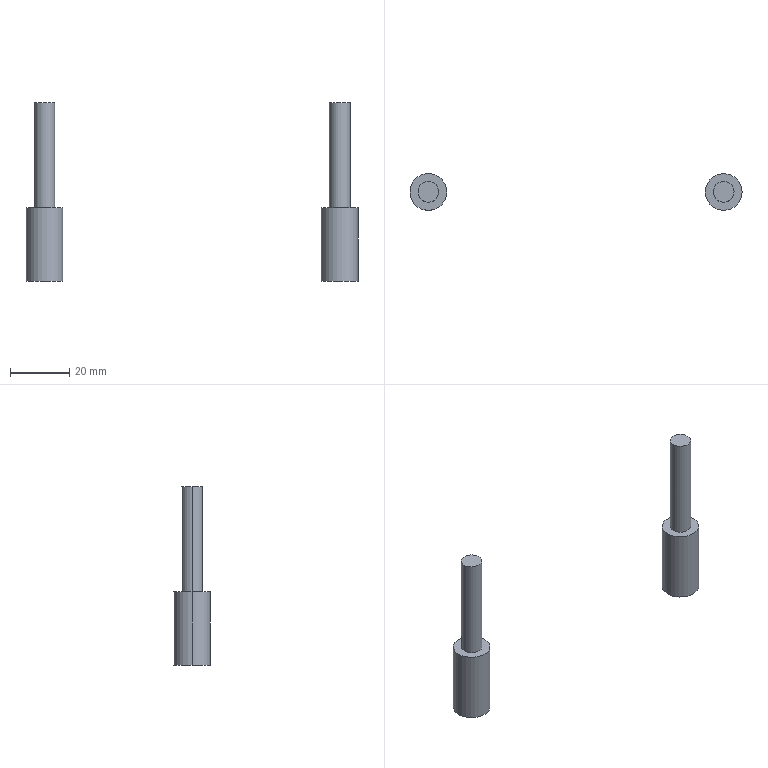Part | STEP file | 吸盘导柱-2 | 2 solids | 14 faces | box 112.418 x 12.438 x 60.6 mm | volume 8796 mm3 | cylinder 8 | plane 6 | commonest cylinder face diameters 7 x4 12.399 x2 12.438 x2
STEP:
#1=CARTESIAN_POINT('',(3.5,0.,60.6));
#2=VERTEX_POINT('',#1);
#3=CARTESIAN_POINT('',(-3.5,0.,60.6));
#4=VERTEX_POINT('',#3);
#5=CARTESIAN_POINT('',(0.,0.,60.6));
#6=DIRECTION('',(0.,0.,1.));
#7=DIRECTION('',(1.,0.,0.));
#8=AXIS2_PLACEMENT_3D('',#5,#6,#7);
#9=CIRCLE('',#8,3.5);
#10=EDGE_CURVE('',#2,#4,#9,.T.);
#11=ORIENTED_EDGE('',*,*,#10,.F.);
#12=CARTESIAN_POINT('',(3.5,0.,25.));
#13=VERTEX_POINT('',#12);
#14=CARTESIAN_POINT('',(3.5,0.,60.6));
#15=DIRECTION('',(0.,0.,-1.));
#16=VECTOR('',#15,1000.);
#17=LINE('',#14,#16);
#18=EDGE_CURVE('',#2,#13,#17,.T.);
#19=ORIENTED_EDGE('',*,*,#18,.T.);
#20=CARTESIAN_POINT('',(-3.5,0.,25.));
#21=VERTEX_POINT('',#20);
#22=CARTESIAN_POINT('',(0.,0.,25.));
#23=DIRECTION('',(0.,0.,1.));
#24=DIRECTION('',(1.,0.,0.));
#25=AXIS2_PLACEMENT_3D('',#22,#23,#24);
#26=CIRCLE('',#25,3.5);
#27=EDGE_CURVE('',#13,#21,#26,.T.);
#28=ORIENTED_EDGE('',*,*,#27,.T.);
#29=CARTESIAN_POINT('',(-3.5,0.,60.6));
#30=DIRECTION('',(0.,0.,-1.));
#31=VECTOR('',#30,1000.);
#32=LINE('',#29,#31);
#33=EDGE_CURVE('',#4,#21,#32,.T.);
#34=ORIENTED_EDGE('',*,*,#33,.F.);
#35=EDGE_LOOP('',(#11,#19,#28,#34));
#36=FACE_OUTER_BOUND('',#35,.T.);
#37=CARTESIAN_POINT('',(0.,0.,60.6));
#38=DIRECTION('',(0.,0.,-1.));
#39=DIRECTION('',(-1.,0.,0.));
#40=AXIS2_PLACEMENT_3D('',#37,#38,#39);
#41=CYLINDRICAL_SURFACE('',#40,3.5);
#42=ADVANCED_FACE('',(#36),#41,.T.);
#43=CARTESIAN_POINT('',(6.219,0.,25.));
#44=VERTEX_POINT('',#43);
#45=CARTESIAN_POINT('',(-6.219,0.,25.));
#46=VERTEX_POINT('',#45);
#47=CARTESIAN_POINT('',(0.,0.,25.));
#48=DIRECTION('',(0.,0.,1.));
#49=DIRECTION('',(1.,0.,0.));
#50=AXIS2_PLACEMENT_3D('',#47,#48,#49);
#51=CIRCLE('',#50,6.219);
#52=EDGE_CURVE('',#44,#46,#51,.T.);
#53=ORIENTED_EDGE('',*,*,#52,.F.);
#54=CARTESIAN_POINT('',(6.219,0.,0.));
#55=VERTEX_POINT('',#54);
#56=CARTESIAN_POINT('',(6.219,0.,25.));
#57=DIRECTION('',(0.,0.,-1.));
#58=VECTOR('',#57,1000.);
#59=LINE('',#56,#58);
#60=EDGE_CURVE('',#44,#55,#59,.T.);
#61=ORIENTED_EDGE('',*,*,#60,.T.);
#62=CARTESIAN_POINT('',(-6.219,0.,0.));
#63=VERTEX_POINT('',#62);
#64=CARTESIAN_POINT('',(0.,0.,0.));
#65=DIRECTION('',(0.,0.,1.));
#66=DIRECTION('',(1.,0.,0.));
#67=AXIS2_PLACEMENT_3D('',#64,#65,#66);
#68=CIRCLE('',#67,6.219);
#69=EDGE_CURVE('',#55,#63,#68,.T.);
#70=ORIENTED_EDGE('',*,*,#69,.T.);
#71=CARTESIAN_POINT('',(-6.219,0.,25.));
#72=DIRECTION('',(0.,0.,-1.));
#73=VECTOR('',#72,1000.);
#74=LINE('',#71,#73);
#75=EDGE_CURVE('',#46,#63,#74,.T.);
#76=ORIENTED_EDGE('',*,*,#75,.F.);
#77=EDGE_LOOP('',(#53,#61,#70,#76));
#78=FACE_OUTER_BOUND('',#77,.T.);
#79=CARTESIAN_POINT('',(0.,0.,25.));
#80=DIRECTION('',(0.,0.,-1.));
#81=DIRECTION('',(-1.,0.,0.));
#82=AXIS2_PLACEMENT_3D('',#79,#80,#81);
#83=CYLINDRICAL_SURFACE('',#82,6.219);
#84=ADVANCED_FACE('',(#78),#83,.T.);
#85=CARTESIAN_POINT('',(0.,0.,25.));
#86=DIRECTION('',(0.,0.,1.));
#87=DIRECTION('',(1.,0.,0.));
#88=AXIS2_PLACEMENT_3D('',#85,#86,#87);
#89=CIRCLE('',#88,6.219);
#90=EDGE_CURVE('',#46,#44,#89,.T.);
#91=ORIENTED_EDGE('',*,*,#90,.T.);
#92=ORIENTED_EDGE('',*,*,#52,.T.);
#93=EDGE_LOOP('',(#91,#92));
#94=FACE_OUTER_BOUND('',#93,.T.);
#95=CARTESIAN_POINT('',(0.,0.,25.));
#96=DIRECTION('',(0.,0.,1.));
#97=DIRECTION('',(1.,0.,0.));
#98=AXIS2_PLACEMENT_3D('',#95,#96,#97);
#99=CIRCLE('',#98,3.5);
#100=EDGE_CURVE('',#21,#13,#99,.T.);
#101=ORIENTED_EDGE('',*,*,#100,.F.);
#102=ORIENTED_EDGE('',*,*,#27,.F.);
#103=EDGE_LOOP('',(#101,#102));
#104=FACE_BOUND('',#103,.T.);
#105=CARTESIAN_POINT('',(0.,0.,25.));
#106=DIRECTION('',(0.,0.,1.));
#107=DIRECTION('',(1.,0.,0.));
#108=AXIS2_PLACEMENT_3D('',#105,#106,#107);
#109=PLANE('',#108);
#110=ADVANCED_FACE('',(#94,#104),#109,.T.);
#111=ORIENTED_EDGE('',*,*,#60,.F.);
#112=ORIENTED_EDGE('',*,*,#90,.F.);
#113=ORIENTED_EDGE('',*,*,#75,.T.);
#114=CARTESIAN_POINT('',(0.,0.,0.));
#115=DIRECTION('',(0.,0.,1.));
#116=DIRECTION('',(1.,0.,0.));
#117=AXIS2_PLACEMENT_3D('',#114,#115,#116);
#118=CIRCLE('',#117,6.219);
#119=EDGE_CURVE('',#63,#55,#118,.T.);
#120=ORIENTED_EDGE('',*,*,#119,.T.);
#121=EDGE_LOOP('',(#111,#112,#113,#120));
#122=FACE_OUTER_BOUND('',#121,.T.);
#123=CARTESIAN_POINT('',(0.,0.,25.));
#124=DIRECTION('',(0.,0.,-1.));
#125=DIRECTION('',(-1.,0.,0.));
#126=AXIS2_PLACEMENT_3D('',#123,#124,#125);
#127=CYLINDRICAL_SURFACE('',#126,6.219);
#128=ADVANCED_FACE('',(#122),#127,.T.);
#129=ORIENTED_EDGE('',*,*,#119,.F.);
#130=ORIENTED_EDGE('',*,*,#69,.F.);
#131=EDGE_LOOP('',(#129,#130));
#132=FACE_OUTER_BOUND('',#131,.T.);
#133=CARTESIAN_POINT('',(0.,0.,0.));
#134=DIRECTION('',(0.,0.,1.));
#135=DIRECTION('',(1.,0.,0.));
#136=AXIS2_PLACEMENT_3D('',#133,#134,#135);
#137=PLANE('',#136);
#138=ADVANCED_FACE('',(#132),#137,.F.);
#139=ORIENTED_EDGE('',*,*,#18,.F.);
#140=CARTESIAN_POINT('',(0.,0.,60.6));
#141=DIRECTION('',(0.,0.,1.));
#142=DIRECTION('',(1.,0.,0.));
#143=AXIS2_PLACEMENT_3D('',#140,#141,#142);
#144=CIRCLE('',#143,3.5);
#145=EDGE_CURVE('',#4,#2,#144,.T.);
#146=ORIENTED_EDGE('',*,*,#145,.F.);
#147=ORIENTED_EDGE('',*,*,#33,.T.);
#148=ORIENTED_EDGE('',*,*,#100,.T.);
#149=EDGE_LOOP('',(#139,#146,#147,#148));
#150=FACE_OUTER_BOUND('',#149,.T.);
#151=CARTESIAN_POINT('',(0.,0.,60.6));
#152=DIRECTION('',(0.,0.,-1.));
#153=DIRECTION('',(-1.,0.,0.));
#154=AXIS2_PLACEMENT_3D('',#151,#152,#153);
#155=CYLINDRICAL_SURFACE('',#154,3.5);
#156=ADVANCED_FACE('',(#150),#155,.T.);
#157=ORIENTED_EDGE('',*,*,#145,.T.);
#158=ORIENTED_EDGE('',*,*,#10,.T.);
#159=EDGE_LOOP('',(#157,#158));
#160=FACE_OUTER_BOUND('',#159,.T.);
#161=CARTESIAN_POINT('',(0.,0.,60.6));
#162=DIRECTION('',(0.,0.,1.));
#163=DIRECTION('',(1.,0.,0.));
#164=AXIS2_PLACEMENT_3D('',#161,#162,#163);
#165=PLANE('',#164);
#166=ADVANCED_FACE('',(#160),#165,.T.);
#167=CLOSED_SHELL('',(#42,#84,#110,#128,#138,#156,#166));
#168=MANIFOLD_SOLID_BREP('',#167);
#169=CARTESIAN_POINT('',(103.5,0.,60.6));
#170=VERTEX_POINT('',#169);
#171=CARTESIAN_POINT('',(96.5,0.,60.6));
#172=VERTEX_POINT('',#171);
#173=CARTESIAN_POINT('',(100.,0.,60.6));
#174=DIRECTION('',(0.,0.,1.));
#175=DIRECTION('',(1.,0.,0.));
#176=AXIS2_PLACEMENT_3D('',#173,#174,#175);
#177=CIRCLE('',#176,3.5);
#178=EDGE_CURVE('',#170,#172,#177,.T.);
#179=ORIENTED_EDGE('',*,*,#178,.F.);
#180=CARTESIAN_POINT('',(103.5,0.,25.));
#181=VERTEX_POINT('',#180);
#182=CARTESIAN_POINT('',(103.5,0.,60.6));
#183=DIRECTION('',(0.,0.,-1.));
#184=VECTOR('',#183,1000.);
#185=LINE('',#182,#184);
#186=EDGE_CURVE('',#170,#181,#185,.T.);
#187=ORIENTED_EDGE('',*,*,#186,.T.);
#188=CARTESIAN_POINT('',(96.5,0.,25.));
#189=VERTEX_POINT('',#188);
#190=CARTESIAN_POINT('',(100.,0.,25.));
#191=DIRECTION('',(0.,0.,1.));
#192=DIRECTION('',(1.,0.,0.));
#193=AXIS2_PLACEMENT_3D('',#190,#191,#192);
#194=CIRCLE('',#193,3.5);
#195=EDGE_CURVE('',#181,#189,#194,.T.);
#196=ORIENTED_EDGE('',*,*,#195,.T.);
#197=CARTESIAN_POINT('',(96.5,0.,60.6));
#198=DIRECTION('',(0.,0.,-1.));
#199=VECTOR('',#198,1000.);
#200=LINE('',#197,#199);
#201=EDGE_CURVE('',#172,#189,#200,.T.);
#202=ORIENTED_EDGE('',*,*,#201,.F.);
#203=EDGE_LOOP('',(#179,#187,#196,#202));
#204=FACE_OUTER_BOUND('',#203,.T.);
#205=CARTESIAN_POINT('',(100.,0.,60.6));
#206=DIRECTION('',(0.,0.,-1.));
#207=DIRECTION('',(-1.,0.,0.));
#208=AXIS2_PLACEMENT_3D('',#205,#206,#207);
#209=CYLINDRICAL_SURFACE('',#208,3.5);
#210=ADVANCED_FACE('',(#204),#209,.T.);
#211=CARTESIAN_POINT('',(106.2,0.,25.));
#212=VERTEX_POINT('',#211);
#213=CARTESIAN_POINT('',(93.8,0.,25.));
#214=VERTEX_POINT('',#213);
#215=CARTESIAN_POINT('',(100.,0.,25.));
#216=DIRECTION('',(0.,0.,1.));
#217=DIRECTION('',(1.,0.,0.));
#218=AXIS2_PLACEMENT_3D('',#215,#216,#217);
#219=CIRCLE('',#218,6.2);
#220=EDGE_CURVE('',#212,#214,#219,.T.);
#221=ORIENTED_EDGE('',*,*,#220,.F.);
#222=CARTESIAN_POINT('',(106.2,0.,0.));
#223=VERTEX_POINT('',#222);
#224=CARTESIAN_POINT('',(106.2,0.,25.));
#225=DIRECTION('',(0.,0.,-1.));
#226=VECTOR('',#225,1000.);
#227=LINE('',#224,#226);
#228=EDGE_CURVE('',#212,#223,#227,.T.);
#229=ORIENTED_EDGE('',*,*,#228,.T.);
#230=CARTESIAN_POINT('',(93.8,0.,0.));
#231=VERTEX_POINT('',#230);
#232=CARTESIAN_POINT('',(100.,0.,0.));
#233=DIRECTION('',(0.,0.,1.));
#234=DIRECTION('',(1.,0.,0.));
#235=AXIS2_PLACEMENT_3D('',#232,#233,#234);
#236=CIRCLE('',#235,6.2);
#237=EDGE_CURVE('',#223,#231,#236,.T.);
#238=ORIENTED_EDGE('',*,*,#237,.T.);
#239=CARTESIAN_POINT('',(93.8,0.,25.));
#240=DIRECTION('',(0.,0.,-1.));
#241=VECTOR('',#240,1000.);
#242=LINE('',#239,#241);
#243=EDGE_CURVE('',#214,#231,#242,.T.);
#244=ORIENTED_EDGE('',*,*,#243,.F.);
#245=EDGE_LOOP('',(#221,#229,#238,#244));
#246=FACE_OUTER_BOUND('',#245,.T.);
#247=CARTESIAN_POINT('',(100.,0.,25.));
#248=DIRECTION('',(0.,0.,-1.));
#249=DIRECTION('',(-1.,0.,0.));
#250=AXIS2_PLACEMENT_3D('',#247,#248,#249);
#251=CYLINDRICAL_SURFACE('',#250,6.2);
#252=ADVANCED_FACE('',(#246),#251,.T.);
#253=CARTESIAN_POINT('',(100.,0.,25.));
#254=DIRECTION('',(0.,0.,1.));
#255=DIRECTION('',(1.,0.,0.));
#256=AXIS2_PLACEMENT_3D('',#253,#254,#255);
#257=CIRCLE('',#256,6.2);
#258=EDGE_CURVE('',#214,#212,#257,.T.);
#259=ORIENTED_EDGE('',*,*,#258,.T.);
#260=ORIENTED_EDGE('',*,*,#220,.T.);
#261=EDGE_LOOP('',(#259,#260));
#262=FACE_OUTER_BOUND('',#261,.T.);
#263=CARTESIAN_POINT('',(100.,0.,25.));
#264=DIRECTION('',(0.,0.,1.));
#265=DIRECTION('',(1.,0.,0.));
#266=AXIS2_PLACEMENT_3D('',#263,#264,#265);
#267=CIRCLE('',#266,3.5);
#268=EDGE_CURVE('',#189,#181,#267,.T.);
#269=ORIENTED_EDGE('',*,*,#268,.F.);
#270=ORIENTED_EDGE('',*,*,#195,.F.);
#271=EDGE_LOOP('',(#269,#270));
#272=FACE_BOUND('',#271,.T.);
#273=CARTESIAN_POINT('',(100.,0.,25.));
#274=DIRECTION('',(0.,0.,1.));
#275=DIRECTION('',(1.,0.,0.));
#276=AXIS2_PLACEMENT_3D('',#273,#274,#275);
#277=PLANE('',#276);
#278=ADVANCED_FACE('',(#262,#272),#277,.T.);
#279=ORIENTED_EDGE('',*,*,#228,.F.);
#280=ORIENTED_EDGE('',*,*,#258,.F.);
#281=ORIENTED_EDGE('',*,*,#243,.T.);
#282=CARTESIAN_POINT('',(100.,0.,0.));
#283=DIRECTION('',(0.,0.,1.));
#284=DIRECTION('',(1.,0.,0.));
#285=AXIS2_PLACEMENT_3D('',#282,#283,#284);
#286=CIRCLE('',#285,6.2);
#287=EDGE_CURVE('',#231,#223,#286,.T.);
#288=ORIENTED_EDGE('',*,*,#287,.T.);
#289=EDGE_LOOP('',(#279,#280,#281,#288));
#290=FACE_OUTER_BOUND('',#289,.T.);
#291=CARTESIAN_POINT('',(100.,0.,25.));
#292=DIRECTION('',(0.,0.,-1.));
#293=DIRECTION('',(-1.,0.,0.));
#294=AXIS2_PLACEMENT_3D('',#291,#292,#293);
#295=CYLINDRICAL_SURFACE('',#294,6.2);
#296=ADVANCED_FACE('',(#290),#295,.T.);
#297=ORIENTED_EDGE('',*,*,#287,.F.);
#298=ORIENTED_EDGE('',*,*,#237,.F.);
#299=EDGE_LOOP('',(#297,#298));
#300=FACE_OUTER_BOUND('',#299,.T.);
#301=CARTESIAN_POINT('',(100.,0.,0.));
#302=DIRECTION('',(0.,0.,1.));
#303=DIRECTION('',(1.,0.,0.));
#304=AXIS2_PLACEMENT_3D('',#301,#302,#303);
#305=PLANE('',#304);
#306=ADVANCED_FACE('',(#300),#305,.F.);
#307=ORIENTED_EDGE('',*,*,#186,.F.);
#308=CARTESIAN_POINT('',(100.,0.,60.6));
#309=DIRECTION('',(0.,0.,1.));
#310=DIRECTION('',(1.,0.,0.));
#311=AXIS2_PLACEMENT_3D('',#308,#309,#310);
#312=CIRCLE('',#311,3.5);
#313=EDGE_CURVE('',#172,#170,#312,.T.);
#314=ORIENTED_EDGE('',*,*,#313,.F.);
#315=ORIENTED_EDGE('',*,*,#201,.T.);
#316=ORIENTED_EDGE('',*,*,#268,.T.);
#317=EDGE_LOOP('',(#307,#314,#315,#316));
#318=FACE_OUTER_BOUND('',#317,.T.);
#319=CARTESIAN_POINT('',(100.,0.,60.6));
#320=DIRECTION('',(0.,0.,-1.));
#321=DIRECTION('',(-1.,0.,0.));
#322=AXIS2_PLACEMENT_3D('',#319,#320,#321);
#323=CYLINDRICAL_SURFACE('',#322,3.5);
#324=ADVANCED_FACE('',(#318),#323,.T.);
#325=ORIENTED_EDGE('',*,*,#313,.T.);
#326=ORIENTED_EDGE('',*,*,#178,.T.);
#327=EDGE_LOOP('',(#325,#326));
#328=FACE_OUTER_BOUND('',#327,.T.);
#329=CARTESIAN_POINT('',(100.,0.,60.6));
#330=DIRECTION('',(0.,0.,1.));
#331=DIRECTION('',(1.,0.,0.));
#332=AXIS2_PLACEMENT_3D('',#329,#330,#331);
#333=PLANE('',#332);
#334=ADVANCED_FACE('',(#328),#333,.T.);
#335=CLOSED_SHELL('',(#210,#252,#278,#296,#306,#324,#334));
#336=MANIFOLD_SOLID_BREP('',#335);
#337=CARTESIAN_POINT('',(0.,0.,0.));
#338=DIRECTION('',(0.,0.,1.));
#339=DIRECTION('',(1.,0.,0.));
#340=AXIS2_PLACEMENT_3D('',#337,#338,#339);
#341=(LENGTH_UNIT()NAMED_UNIT(*)SI_UNIT(.MILLI.,.METRE.));
#342=UNCERTAINTY_MEASURE_WITH_UNIT(LENGTH_MEASURE(0.00001),#341,'','');
#343=(NAMED_UNIT(*)PLANE_ANGLE_UNIT()SI_UNIT($,.RADIAN.));
#344=(NAMED_UNIT(*)SI_UNIT($,.STERADIAN.)SOLID_ANGLE_UNIT());
#345=(GEOMETRIC_REPRESENTATION_CONTEXT(3)GLOBAL_UNCERTAINTY_ASSIGNED_CONTEXT((#342))GLOBAL_UNIT_ASSIGNED_CONTEXT((#341,#343,#344))REPRESENTATION_CONTEXT('',''));
#346=ADVANCED_BREP_SHAPE_REPRESENTATION('',(#168,#336,#340),#345);